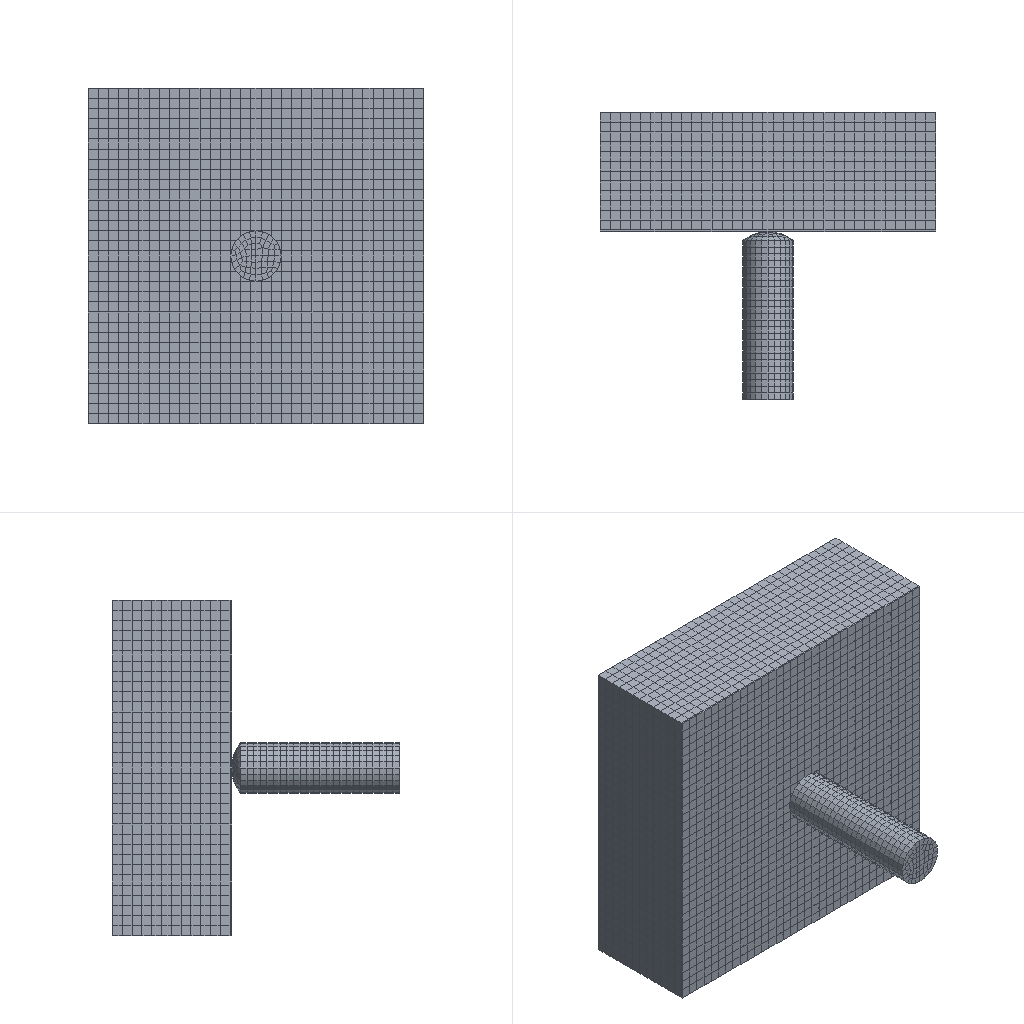Simulation study | abaqus
Set-up summary:
category,name,step,type,value,unit,region
solver,abaqus
solver,version,,,Abaqus/Standard 2020
units,not stated in the deck,,not stated
analysis,deck,,static,static
load_step,Step-1,Step-1,static,nlgeom=True
contact,interactions,,,general=1 pairs=0 ties=0
load_step,requested,,,1
mesh,nodes,,,19215
mesh,elements,,,15645
element_type,C3D8R,,solid,15645
load,load commands in deck,,count,1
bc,support commands in deck,,count,6
material,JINGPIAN,,in results
material,LV,,in results
material,ZHEN,,in results
check,setup vs results,,match,"per instance, exact: element labels, types and connectivity; labels of the nodes the elements use; coordinates of those nodes at SINGLE_PRECISION in 2 of 3 instance(s)"
Abaqus input file, long lists of numbers shortened:
*Heading
** Job name: Job-1 Model name: Model-1
** Generated by: Abaqus/CAE 2020
*Preprint, echo=NO, model=NO, history=NO, contact=NO
**
** PARTS
**
*Part, name=work-1
*Node
      1,         -0.5, 0.0045,         -0.5
      2,         -0.5, 0.0045, -0.4697
** (15026 more lines like these left out)
*Element, type=C3D8R
    1,   443,   444,   478,   477,     1,     2,    36,    35
    2,   444,   445,   479,   478,     2,     3,    37,    36
** (13066 more lines like these left out)
*Nset, nset=Set-1, generate
     1,  15028,      1
*Elset, elset=Set-1, generate
     1,  13068,      1
** Section: jing
*Solid Section, elset=Set-1, material=jingpian
,
*End Part
**
*Part, name=work-2
*Node
      1,         -0.5,           0.,         -0.5
      2,         -0.5,           0., -0.4697
** (2310 more lines like these left out)
*Element, type=C3D8R
   1,   69,   70,  104,  103,    1,    2,   36,   35
   2,   70,   71,  105,  104,    2,    3,   37,   36
** (1087 more lines like these left out)
*Nset, nset=Set-1, generate
    1,  2312,     1
*Elset, elset=Set-1, generate
    1,  1089,     1
** Section: lv
*Solid Section, elset=Set-1, material=lv
,
*End Part
**
*Part, name=zhen
*Node
      1,           0.,           0.,           0.
      2,           0., -0.075, -0.02633
** (1873 more lines like these left out)
*Element, type=C3D8R
   1,   39,    9,    2,    8,  114,   84,   77,   83
   2,   38,   10,    9,   39,  113,   85,   84,  114
** (1486 more lines like these left out)
*Nset, nset=Set-1, generate
    1,  1875,     1
*Elset, elset=Set-1, generate
    1,  1488,     1
** Section: zhen
*Solid Section, elset=Set-1, material=zhen
,
*End Part
**
**
** ASSEMBLY
**
*Assembly, name=Assembly
**
*Instance, name=work-1-1, part=work-1
*End Instance
**
*Instance, name=work-2-1, part=work-2
*End Instance
**
*Instance, name=zhen-1, part=zhen
          0.,           0.,           0.
          0.,           0.,           0., -1.,           0.,           0., 90.
*End Instance
**
*Node
      1,           0.,         -0.5, -3.52085954e-17
*Nset, nset=Set-1, instance=work-1-1
   409,   410,   411,   412,   413,   414,   415,   416,   417,   418,   419,   420,   421,   422,   423,   424
   425,   426,   427,   428,   429,   430,   431,   432,   433,   434,   435,   436,   437,   438,   439,   440
** (71 more lines like these left out)
*Elset, elset=Set-1, instance=work-1-1
   364,   365,   366,   367,   368,   369,   370,   371,   372,   373,   374,   375,   376,   377,   378,   379
   380,   381,   382,   383,   384,   385,   386,   387,   388,   389,   390,   391,   392,   393,   394,   395
** (67 more lines like these left out)
*Nset, nset=Set-4, instance=zhen-1, generate
    1,  1875,     1
*Elset, elset=Set-4, instance=zhen-1, generate
    1,  1488,     1
*Nset, nset=Set-5
 1,
*Nset, nset=b_Set-2, instance=zhen-1, generate
    1,  1875,     1
*Elset, elset=b_Set-2, instance=zhen-1, generate
    1,  1488,     1
*Nset, nset=_PickedSet11, internal
 1,
** Constraint: Constraint-1
*Rigid Body, ref node=_PickedSet11, elset=b_Set-2
*Elset, elset=__Int-1_gcs0_13_S3, internal, instance=zhen-1
    6,   52,   56,   68,  114,  118,  130,  176,  180,  192,  238,  242,  254,  300,  304,  316
  362,  366,  378,  424,  428,  440,  486,  490,  502,  548,  552,  564,  610,  614,  626,  672
** (3 more lines like these left out)
*Elset, elset=__Int-1_gcs0_13_S4, internal, instance=zhen-1
    7,   19,   31,   69,   81,   93,  131,  143,  155,  193,  205,  217,  255,  267,  279,  317
  329,  341,  379,  391,  403,  441,  453,  465,  503,  515,  527,  565,  577,  589,  627,  639
** (3 more lines like these left out)
*Elset, elset=__Int-1_gcs0_13_S6, internal, instance=zhen-1
    9,   20,   23,   30,   61,   71,   82,   85,   92,  123,  133,  144,  147,  154,  185,  195
  206,  209,  216,  247,  257,  268,  271,  278,  309,  319,  330,  333,  340,  371,  381,  392
** (6 more lines like these left out)
*Elset, elset=__Int-1_gcs0_13_S5, internal, instance=zhen-1, generate
   59,  1485,    62
*Surface, type=ELEMENT, name=_Int-1_gcs0_13, internal
__Int-1_gcs0_13_S3, S3
__Int-1_gcs0_13_S4, S4
__Int-1_gcs0_13_S6, S6
__Int-1_gcs0_13_S5, S5
*Elset, elset=__Int-1_gcs0_14_S1, internal, instance=zhen-1, generate
 30,  62,   1
*Surface, type=ELEMENT, name=_Int-1_gcs0_14, internal
__Int-1_gcs0_14_S1, S1
*Elset, elset=__Int-1_gcs0_15_S1, internal, instance=zhen-1, generate
  1,  29,   1
*Surface, type=ELEMENT, name=_Int-1_gcs0_15, internal
__Int-1_gcs0_15_S1, S1
*Elset, elset=__Int-1_gcs0_17_S4, internal, instance=zhen-1
    1,    2,   16,   21,   22,   63,   64,   78,   83,   84,  125,  126,  140,  145,  146,  187
  188,  202,  207,  208,  249,  250,  264,  269,  270,  311,  312,  326,  331,  332,  373,  374
** (6 more lines like these left out)
*Elset, elset=__Int-1_gcs0_17_S6, internal, instance=zhen-1, generate
   24,  1450,    62
*Elset, elset=__Int-1_gcs0_17_S5, internal, instance=zhen-1, generate
   34,  1460,    62
*Elset, elset=__Int-1_gcs0_17_S3, internal, instance=zhen-1
   37,   43,   44,   55,   58,   99,  105,  106,  117,  120,  161,  167,  168,  179,  182,  223
  229,  230,  241,  244,  285,  291,  292,  303,  306,  347,  353,  354,  365,  368,  409,  415
** (6 more lines like these left out)
*Surface, type=ELEMENT, name=_Int-1_gcs0_17, internal
__Int-1_gcs0_17_S4, S4
__Int-1_gcs0_17_S6, S6
__Int-1_gcs0_17_S5, S5
__Int-1_gcs0_17_S3, S3
*End Assembly
*Amplitude, name=Amp-1
             0.,              0.,              1.,              1.
**
** MATERIALS
**
*Material, name=jingpian
*Density
 3.2e-09,
*Elastic
480000., 0.215
*Material, name=lv
*Density
 3.9e-09,
*Elastic
350000., 0.25
*Material, name=zhen
*Density
 8.36e-09,
*Elastic
131000., 0.3
**
** INTERACTION PROPERTIES
**
*Surface Interaction, name=IntProp-1
1.,
*Friction, slip tolerance=0.005
 0.2,
*Surface Behavior, pressure-overclosure=HARD
**
** INTERACTIONS
**
** Interaction: Int-1
*Contact
*Contact Inclusions, ALL EXTERIOR
*Contact Property Assignment
 ,  , IntProp-1
*Surface Property Assignment, property=GEOMETRIC CORRECTION
_Int-1_gcs0_13, Circumferential, 0., 0.04722, 2.8911e-18,  0., -0.9528, -5.83412e-17
_Int-1_gcs0_14, Spherical, 0., -0.12, 1.82973e-17
_Int-1_gcs0_15, Spherical, 0., -0.12, 1.82973e-17
_Int-1_gcs0_17, Circumferential, 0., 0.04722, 2.8911e-18,  0., -0.9528, -5.83412e-17
** ----------------------------------------------------------------
**
** STEP: Step-1
**
*Step, name=Step-1, nlgeom=YES, inc=1000
*Static, stabilize=0.0002, allsdtol=0.05, continue=NO
0.01, 1., 1e-05, 1.
**
** BOUNDARY CONDITIONS
**
** Name: BC-1 Type: 对称/反对称/完全固定
*Boundary
Set-1, ENCASTRE
** Name: BC-2 Type: 位移/转角
*Boundary
Set-5, 1, 1
Set-5, 3, 3
Set-5, 4, 4
Set-5, 5, 5
Set-5, 6, 6
**
** LOADS
**
** Name: Load-1   Type: Gravity
*Dload, amplitude=Amp-1
Set-4, GRAV, 196000., 0., 1., 0.
**
** OUTPUT REQUESTS
**
*Restart, write, frequency=0
**
** FIELD OUTPUT: F-Output-1
**
*Output, field
*Node Output
CF, RF, RM, RT, TF, U, V
*Element Output, directions=YES
E, LE, MISES, MISESMAX, NE, PE, PEEQ, PEEQMAX, PEEQT, PEMAG, S, SEQUT, SF, VEEQ, YIELDPOT
*Contact Output
CDISP, CSTRESS
**
** HISTORY OUTPUT: H-Output-1
**
*Output, history, variable=PRESELECT
*End Step
Results summary:
result,step,,completed,increments=14 time=1.0/1.0
result,analysis,,,static
result,last_loadstep,,,1
result,analysis steps,,count,1
result,primary field,,,U
result,reaction total,,FX,0.0,model units
result,reaction total,,FY,-1.4e-05,model units
result,reaction total,,FZ,0.0,model units